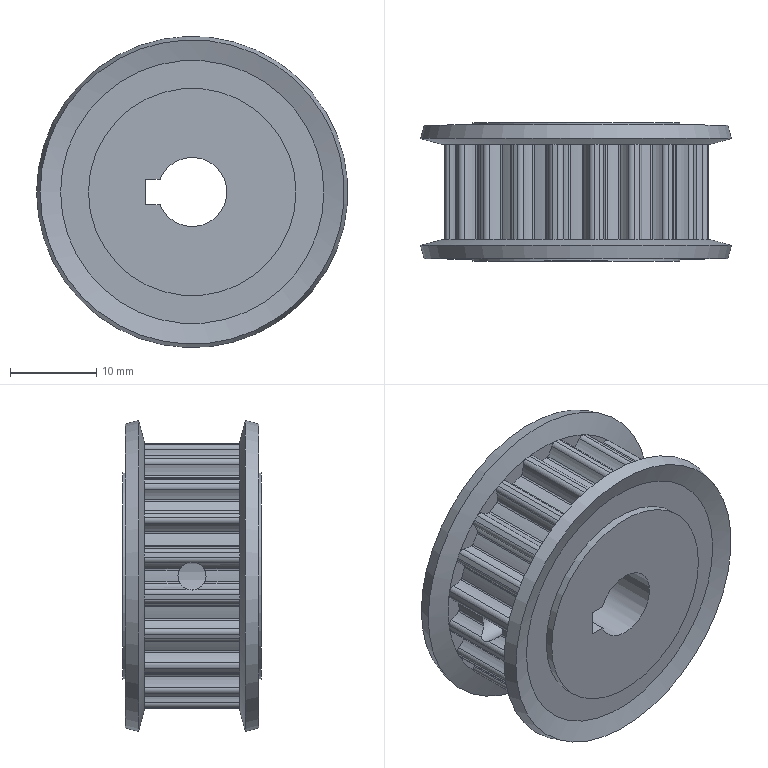Part | STEP file | ROTATION MC_NEW VER-0610_477 | 1 solid | 231 faces | box 36 x 16 x 36 mm | volume 10187 mm3 | cylinder 175 | plane 50 | cone 6 | commonest cylinder face diameters 0.5 x44 6.55 x44 1.1 x40 27.33 x22 30.87 x20 3.242 x2